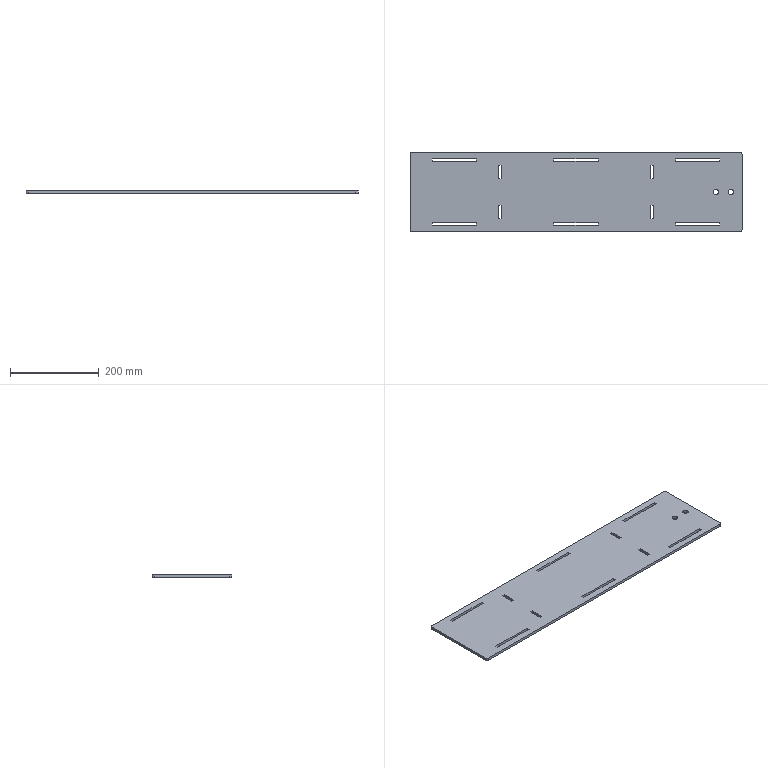Part | SolidWorks | features FlatPattern 1, SMBaseFlange 1, SheetMetal 1 | 1 solid | 54 faces | box 750 x 180 x 6 mm | volume 782502 mm3 | plane 46 | cylinder 8 | commonest cylinder face diameters 10 x4 12.4 x4